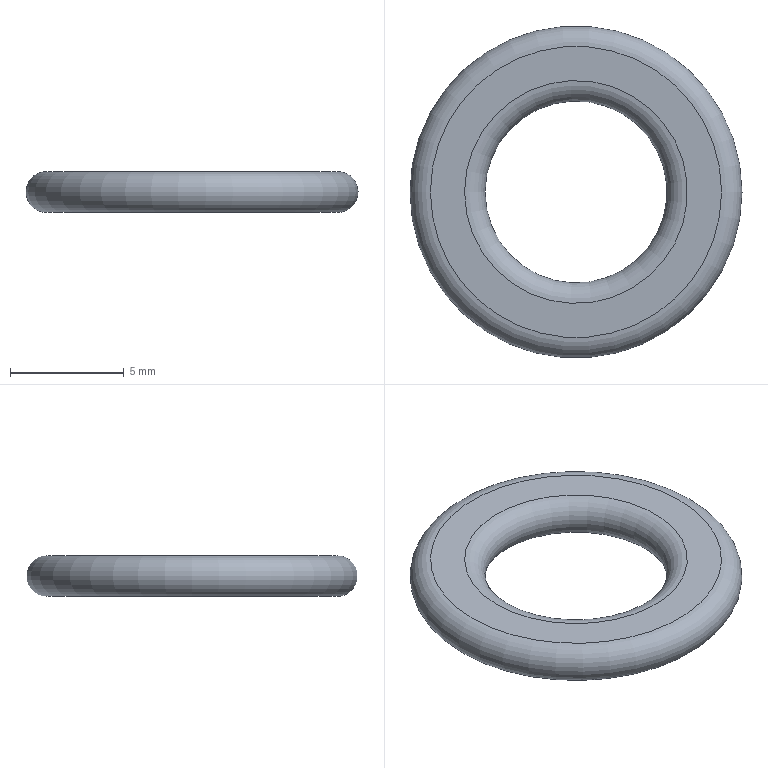Part | NX | features solid 2 | 1 solid | 4 faces | box 14.6 x 14.6 x 1.8 mm | volume 186.186 mm3 | plane 2 | torus 2
STEP:
#1=CARTESIAN_POINT('',(80.1,35.,-130.));
#2=VERTEX_POINT('',#1);
#3=CARTESIAN_POINT('',(85.,35.,-130.));
#4=DIRECTION('',(0.,0.,-1.));
#5=DIRECTION('',(-1.,0.,0.));
#6=AXIS2_PLACEMENT_3D('',#3,#4,#5);
#7=CIRCLE('',#6,4.9);
#8=EDGE_CURVE('',#2,#2,#7,.T.);
#9=ORIENTED_EDGE('',*,*,#8,.T.);
#10=EDGE_LOOP('',(#9));
#11=FACE_BOUND('',#10,.T.);
#12=CARTESIAN_POINT('',(78.6,35.,-130.));
#13=VERTEX_POINT('',#12);
#14=CARTESIAN_POINT('',(85.,35.,-130.));
#15=DIRECTION('',(0.,0.,-1.));
#16=DIRECTION('',(-1.,0.,0.));
#17=AXIS2_PLACEMENT_3D('',#14,#15,#16);
#18=CIRCLE('',#17,6.4);
#19=EDGE_CURVE('',#13,#13,#18,.T.);
#20=ORIENTED_EDGE('',*,*,#19,.F.);
#21=EDGE_LOOP('',(#20));
#22=FACE_BOUND('',#21,.T.);
#23=CARTESIAN_POINT('',(91.4,35.,-130.));
#24=DIRECTION('',(0.,0.,1.));
#25=DIRECTION('',(1.,0.,0.));
#26=AXIS2_PLACEMENT_3D('',#23,#24,#25);
#27=PLANE('',#26);
#28=ADVANCED_FACE('',(#11,#22),#27,.T.);
#29=CARTESIAN_POINT('',(80.1,35.,-131.8));
#30=VERTEX_POINT('',#29);
#31=CARTESIAN_POINT('',(85.,35.,-131.8));
#32=DIRECTION('',(0.,0.,-1.));
#33=DIRECTION('',(-1.,0.,0.));
#34=AXIS2_PLACEMENT_3D('',#31,#32,#33);
#35=CIRCLE('',#34,4.9);
#36=EDGE_CURVE('',#30,#30,#35,.T.);
#37=ORIENTED_EDGE('',*,*,#36,.T.);
#38=EDGE_LOOP('',(#37));
#39=FACE_BOUND('',#38,.T.);
#40=ORIENTED_EDGE('',*,*,#8,.F.);
#41=EDGE_LOOP('',(#40));
#42=FACE_BOUND('',#41,.T.);
#43=CARTESIAN_POINT('',(85.,35.,-130.9));
#44=DIRECTION('',(0.,0.,-1.));
#45=DIRECTION('',(-1.,0.,0.));
#46=AXIS2_PLACEMENT_3D('',#43,#44,#45);
#47=TOROIDAL_SURFACE('',#46,4.9,0.9);
#48=ADVANCED_FACE('',(#39,#42),#47,.T.);
#49=CARTESIAN_POINT('',(78.6,35.,-131.8));
#50=VERTEX_POINT('',#49);
#51=CARTESIAN_POINT('',(85.,35.,-131.8));
#52=DIRECTION('',(0.,0.,-1.));
#53=DIRECTION('',(-1.,0.,0.));
#54=AXIS2_PLACEMENT_3D('',#51,#52,#53);
#55=CIRCLE('',#54,6.4);
#56=EDGE_CURVE('',#50,#50,#55,.T.);
#57=ORIENTED_EDGE('',*,*,#56,.T.);
#58=EDGE_LOOP('',(#57));
#59=FACE_BOUND('',#58,.T.);
#60=ORIENTED_EDGE('',*,*,#36,.F.);
#61=EDGE_LOOP('',(#60));
#62=FACE_BOUND('',#61,.T.);
#63=CARTESIAN_POINT('',(89.9,35.,-131.8));
#64=DIRECTION('',(0.,0.,-1.));
#65=DIRECTION('',(-1.,0.,0.));
#66=AXIS2_PLACEMENT_3D('',#63,#64,#65);
#67=PLANE('',#66);
#68=ADVANCED_FACE('',(#59,#62),#67,.T.);
#69=ORIENTED_EDGE('',*,*,#19,.T.);
#70=EDGE_LOOP('',(#69));
#71=FACE_BOUND('',#70,.T.);
#72=ORIENTED_EDGE('',*,*,#56,.F.);
#73=EDGE_LOOP('',(#72));
#74=FACE_BOUND('',#73,.T.);
#75=CARTESIAN_POINT('',(85.,35.,-130.9));
#76=DIRECTION('',(0.,0.,-1.));
#77=DIRECTION('',(-1.,0.,0.));
#78=AXIS2_PLACEMENT_3D('',#75,#76,#77);
#79=TOROIDAL_SURFACE('',#78,6.4,0.9);
#80=ADVANCED_FACE('',(#71,#74),#79,.T.);
#81=CLOSED_SHELL('',(#28,#48,#68,#80));
#82=MANIFOLD_SOLID_BREP('',#81);
#83=(LENGTH_UNIT()NAMED_UNIT(*)SI_UNIT(.MILLI.,.METRE.));
#84=UNCERTAINTY_MEASURE_WITH_UNIT(LENGTH_MEASURE(0.00001),#83,'','');
#85=(NAMED_UNIT(*)PLANE_ANGLE_UNIT()SI_UNIT($,.RADIAN.));
#86=(NAMED_UNIT(*)SI_UNIT($,.STERADIAN.)SOLID_ANGLE_UNIT());
#87=(GEOMETRIC_REPRESENTATION_CONTEXT(3)GLOBAL_UNCERTAINTY_ASSIGNED_CONTEXT((#84))GLOBAL_UNIT_ASSIGNED_CONTEXT((#83,#85,#86))REPRESENTATION_CONTEXT('',''));
#88=ADVANCED_BREP_SHAPE_REPRESENTATION('',(#82),#87);